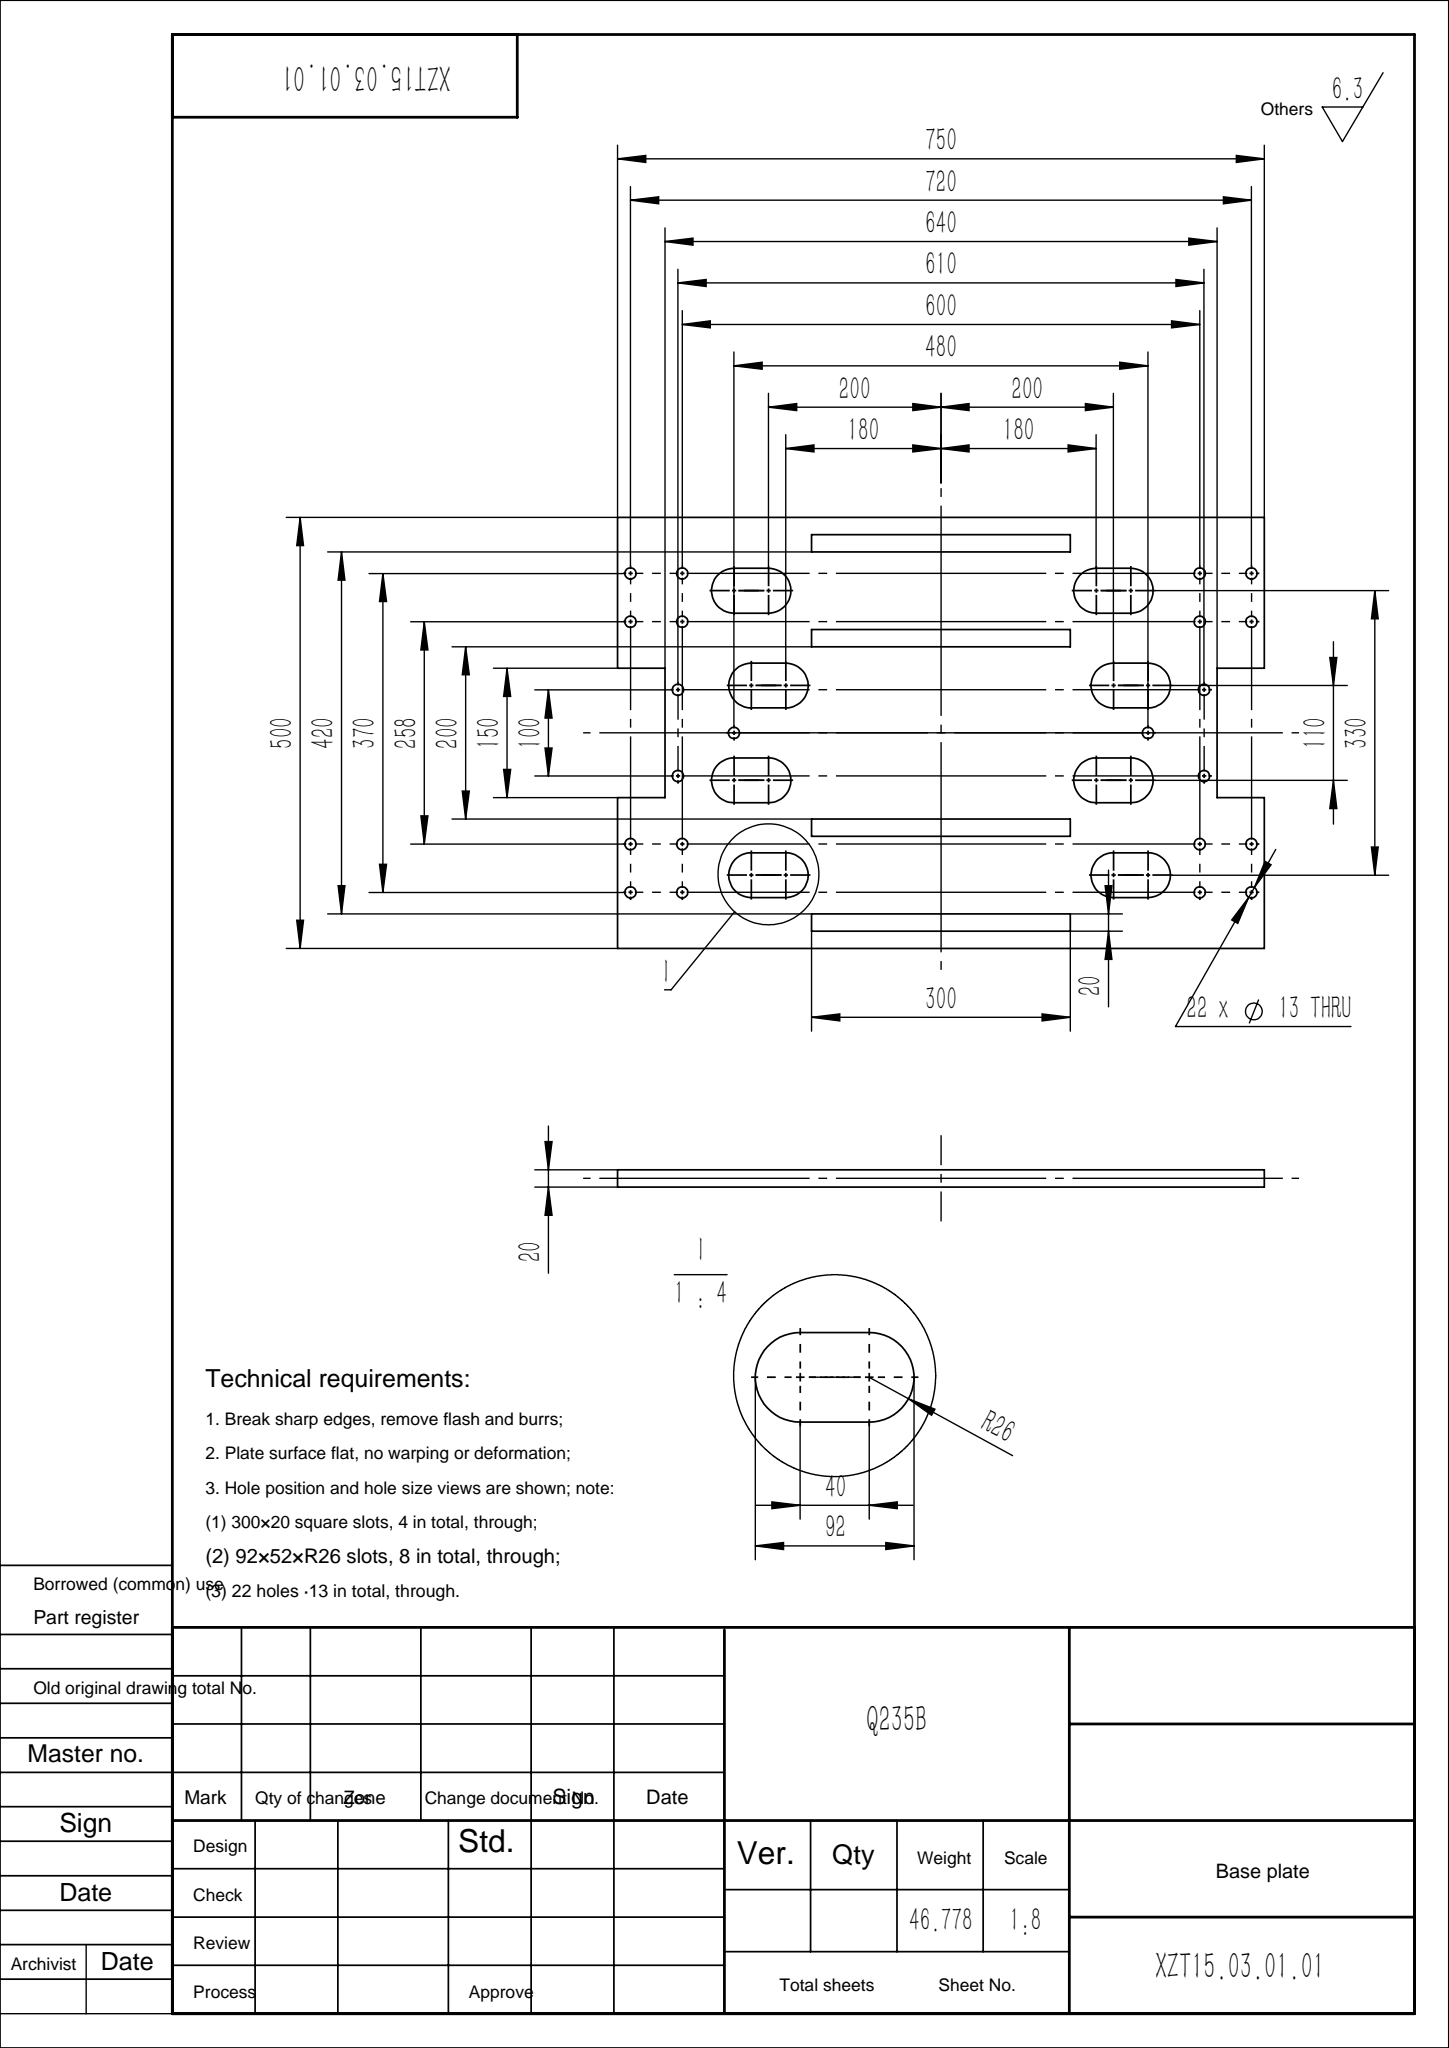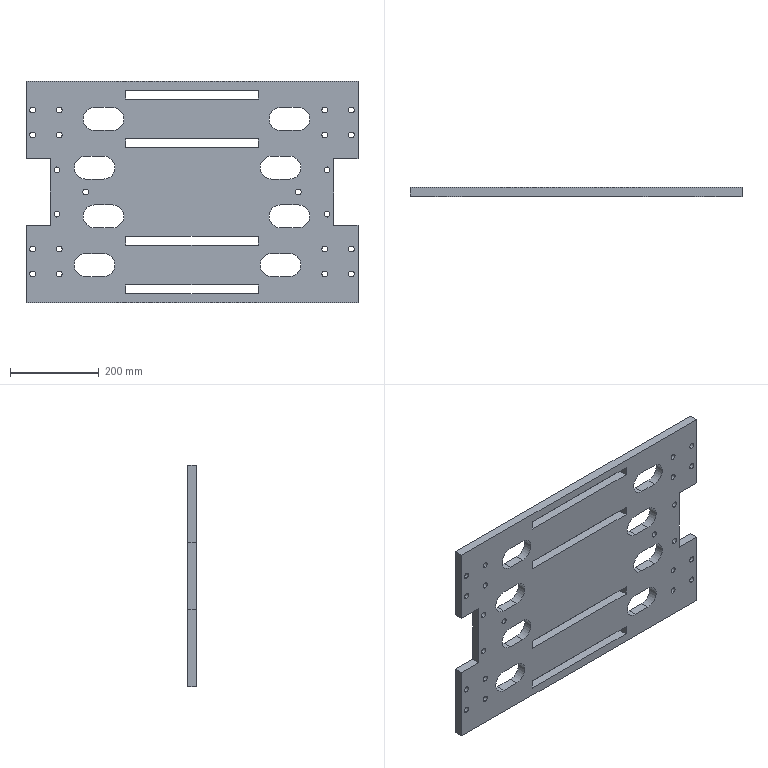Part | SolidWorks | features Extrusion 1, HoleWzd 1, ICE 1 | 1 solid | 106 faces | box 750 x 20 x 500 mm | volume 5959003 mm3 | cylinder 60 | plane 46 | commonest cylinder face diameters 13 x44 52 x16